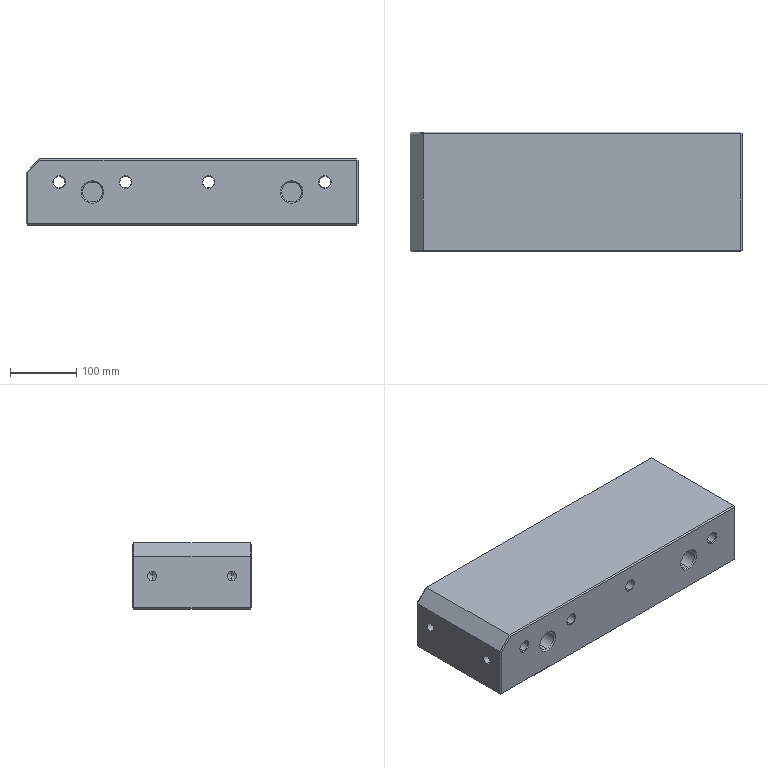Part | STEP file | Spacer block 02 - Tower - 1 cav | 1 solid | 86 faces | box 500 x 180 x 100 mm | volume 8645281 mm3 | cone 32 | plane 30 | cylinder 24 | commonest cylinder face diameters 14 x8 17 x8 30 x8